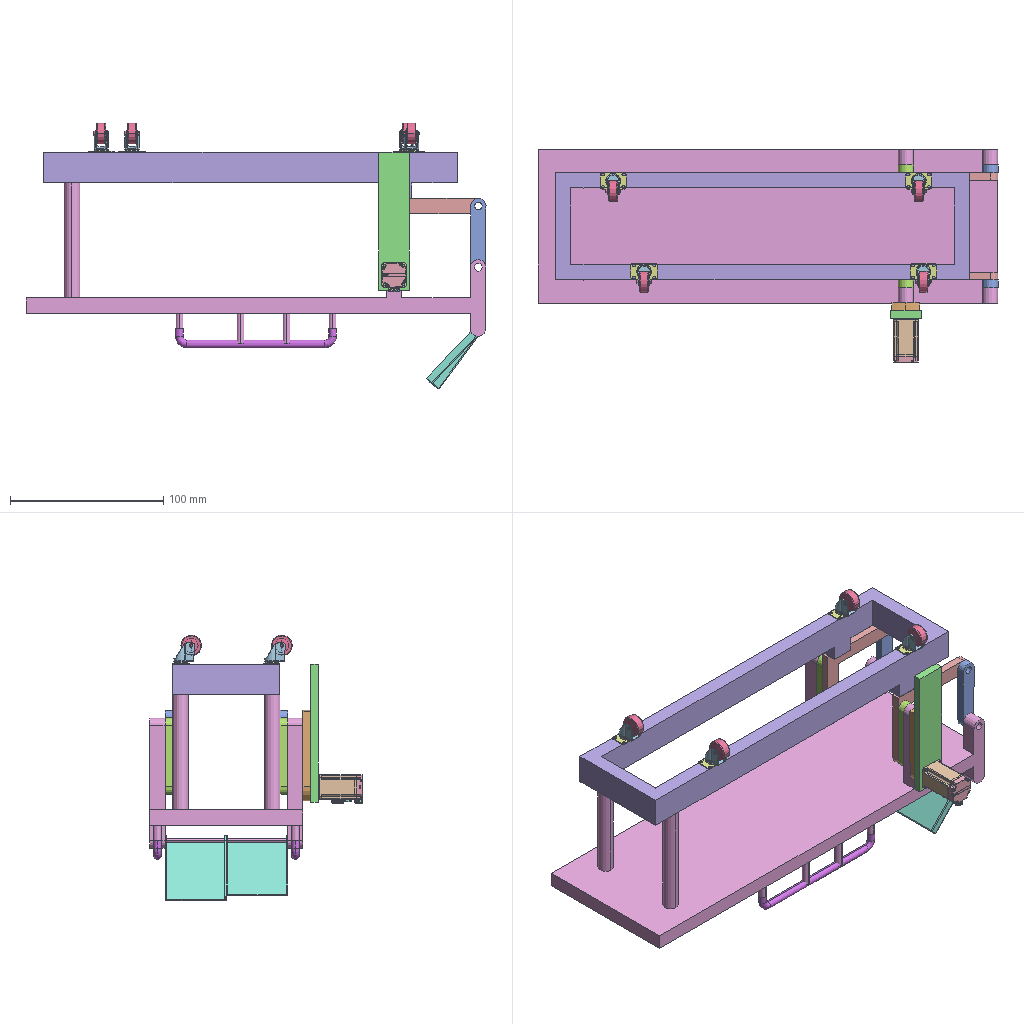Assembly | SolidWorks | 11 different items | 19 placed | box 300 x 139 x 173 mm
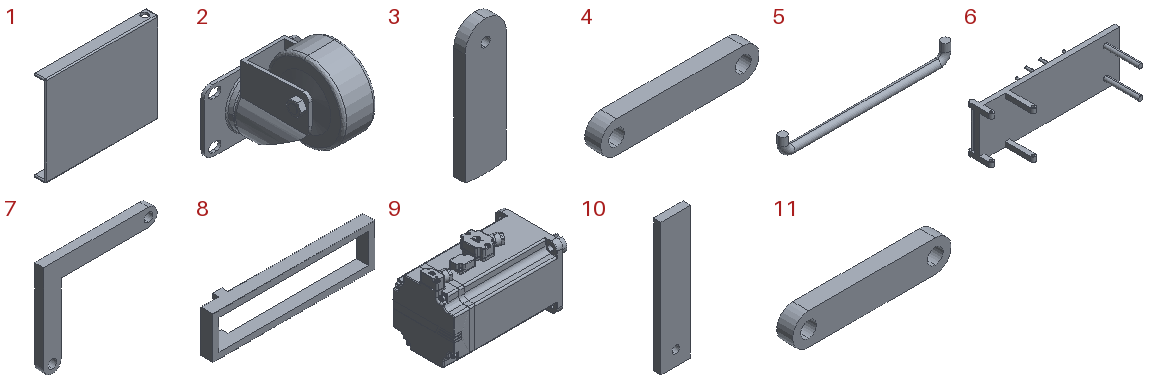Parts list (item | quantity | size | volume | features):
1 | x2 | 50 x 5 x 40 mm | 2370 mm3 | features ICE 2, Extrusion 1, Fillet 1, MirrorPattern 1, MoveFace 1
2 | x4 | 17.1 x 19.08 x 18.81 mm | 1198 mm3 | features ICE 4, BaseBody 2, Fillet 2, Extrusion 1, Revolution 1, Scale 1
3 | x1 | 18.129 x 10 x 59.065 mm | 5188 mm3 | features ICE 3, Extrusion 1
4 | x2 | 50 x 5 x 10 mm | 2196 mm3 | features Extrusion 1
5 | x2 | 105 x 5 x 12.5 mm | 2272 mm3 | features Sweep 1
6 | x1 | 300 x 105 x 100 mm | 333273 mm3 | features ICE 7, MirrorPattern 2, Extrusion 1, Fillet 1
7 | x2 | 65 x 5 x 55 mm | 5196 mm3 | features Extrusion 1
8 | x1 | 270 x 30 x 70 mm | 131000 mm3 | features Extrusion 1, ICE 1, MoveFace 1
9 | x1 | - | - | features RefSurface 87, BaseBody 3, MoveFace 2, Scale 1
10 | x1 | 20 x 5 x 90 mm | 8902 mm3 | features Extrusion 1
11 | x2 | 50 x 5 x 10 mm | 2196 mm3 | features Extrusion 1
Mates (type | each side: item.copy, entity, surface, feature):
Concentric | 7.1 face cylinder Boss-Extrude1 | 4.1 face cylinder Boss-Extrude1
Coincident | 7.1 face plane Boss-Extrude1 | 4.1 face plane Boss-Extrude1
Concentric | 7.1 face cylinder Boss-Extrude1 | 11.1 face cylinder Boss-Extrude1
Coincident | 7.1 face plane Boss-Extrude1 | 11.1 face plane Boss-Extrude1
Concentric | 4.1 face cylinder Boss-Extrude1 | 6.1 face cylinder Boss-Extrude2
Coincident | 4.1 face plane Boss-Extrude1 | 6.1 face plane Boss-Extrude2
Concentric | 11.1 face cylinder Boss-Extrude1 | 6.1 face cylinder Boss-Extrude2
Coincident | 7.1 face plane Boss-Extrude1 | 7.2 face plane Boss-Extrude1 | 2 times
Coincident | 6.1 face plane Mirror1 | 4.2 face plane Boss-Extrude1
Concentric | 6.1 face cylinder Mirror1 | 4.2 face cylinder Boss-Extrude1
Concentric | 7.2 face cylinder Boss-Extrude1 | 4.2 face cylinder Boss-Extrude1
Coincident | 7.2 face plane Boss-Extrude1 | 4.2 face plane Boss-Extrude1
Concentric | 7.2 face cylinder Boss-Extrude1 | 11.2 face cylinder Boss-Extrude1
Coincident | 7.2 face plane Boss-Extrude1 | 11.2 face plane Boss-Extrude1
Concentric | 6.1 face cylinder Mirror1 | 11.2 face cylinder Boss-Extrude1
Parallel | 6.1 face plane Mirror1 | 11.2 face plane Boss-Extrude1
Concentric | 6.1 face cylinder Boss-Extrude4 | 1.1 face cylinder Cut-Extrude1
Coincident | 6.1 face plane Boss-Extrude3 | 1.1 face plane Boss-Extrude1
Concentric | 6.1 face cylinder Boss-Extrude4 | 1.2 face cylinder Cut-Extrude1
Coincident | 1.1 face plane Boss-Extrude1 | 1.2 face plane Boss-Extrude1
Concentric | 11.1 face cylinder Boss-Extrude1 | 3.1 face cylinder Boss-Extrude1
Concentric | 6.1 face cylinder Boss-Extrude2 | 3.1 face cylinder Boss-Extrude2
Coincident | 6.1 face plane Boss-Extrude1 | 3.1 face plane Boss-Extrude1
Coincident | 7.1 face plane Boss-Extrude1 | 8.1 face plane Boss-Extrude2
Coincident | 7.1 face plane Boss-Extrude1 | 8.1 face plane Boss-Extrude1
Concentric | 3.1 face cylinder Cut-Extrude2 | 9.1 face cylinder Surface-Input 13
Parallel | 7.1 face plane Boss-Extrude1 | 9.1 face plane Surface-Input 12
Concentric | 3.1 face cylinder Cut-Extrude2 | 10.1 face cylinder Boss-Extrude1
Parallel | 8.1 face plane Boss-Extrude1 | 10.1 face plane Boss-Extrude1
Coincident | 3.1 face plane Boss-Extrude1 | 10.1 face plane Boss-Extrude1
Coincident | 9.1 face plane Surface-Input 12 | 10.1 face plane Boss-Extrude1
Coincident | 8.1 face plane Boss-Extrude1 | 2.1 face plane Boss-Extrude1 | 2 times
Coincident | 8.1 face plane Boss-Extrude1 | 2.2 face plane Boss-Extrude1 | 2 times
Coincident | 8.1 face plane Boss-Extrude1 | 2.3 face plane Boss-Extrude1 | 2 times
Coincident | 8.1 face plane Boss-Extrude1 | 2.4 face plane Boss-Extrude1 | 2 times
Concentric | 6.1 face cylinder Boss-Extrude6 | 5.1 face cylinder Sweep1 | 2 times
Coincident | 6.1 face plane Boss-Extrude6 | 5.1 face plane Sweep1
Concentric | 6.1 face cylinder Boss-Extrude6 | 5.2 face cylinder Sweep1 | 2 times
Coincident | 6.1 face plane Boss-Extrude6 | 5.2 face plane Sweep1